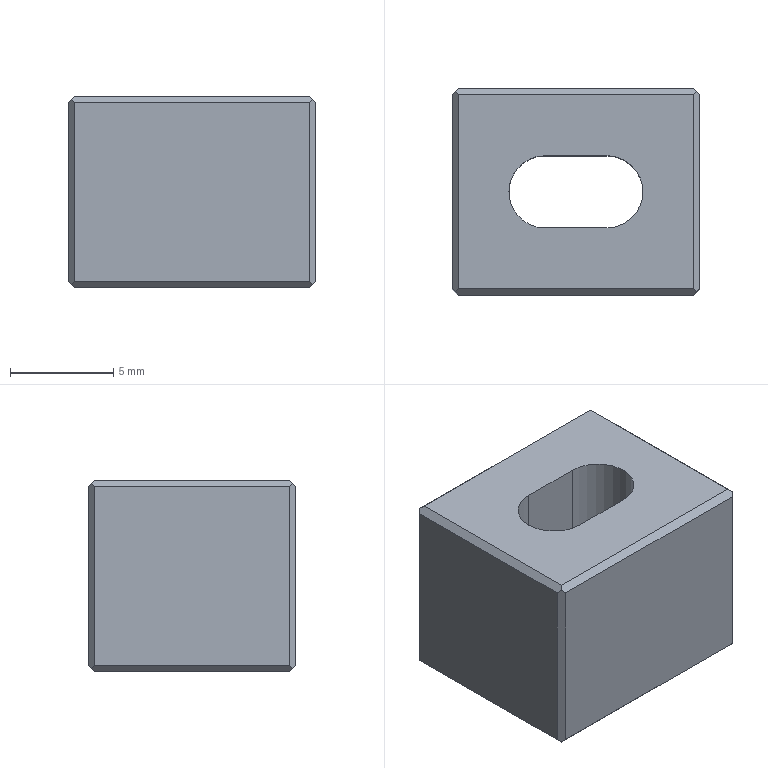Part | NX | 1 solid | 23 faces | box 12 x 10 x 9.3 mm | volume 923.402 mm3 | plane 20 | cylinder 3 | commonest cylinder face diameters 3.5 x3
STEP:
#1=CARTESIAN_POINT('',(-158.2,155.,-51.9));
#2=VERTEX_POINT('',#1);
#3=CARTESIAN_POINT('',(-146.8,155.,-51.9));
#4=VERTEX_POINT('',#3);
#5=CARTESIAN_POINT('',(-152.35,155.,-51.9));
#6=DIRECTION('',(1.,0.,0.));
#7=VECTOR('',#6,1000.);
#8=LINE('',#5,#7);
#9=EDGE_CURVE('',#2,#4,#8,.T.);
#10=ORIENTED_EDGE('',*,*,#9,.T.);
#11=CARTESIAN_POINT('',(-146.8,155.,-43.2));
#12=VERTEX_POINT('',#11);
#13=CARTESIAN_POINT('',(-146.8,155.,-47.55));
#14=DIRECTION('',(0.,0.,1.));
#15=VECTOR('',#14,1000.);
#16=LINE('',#13,#15);
#17=EDGE_CURVE('',#4,#12,#16,.T.);
#18=ORIENTED_EDGE('',*,*,#17,.T.);
#19=CARTESIAN_POINT('',(-158.2,155.,-43.2));
#20=VERTEX_POINT('',#19);
#21=CARTESIAN_POINT('',(-152.5,155.,-43.2));
#22=DIRECTION('',(1.,0.,0.));
#23=VECTOR('',#22,1000.);
#24=LINE('',#21,#23);
#25=EDGE_CURVE('',#20,#12,#24,.T.);
#26=ORIENTED_EDGE('',*,*,#25,.F.);
#27=CARTESIAN_POINT('',(-158.2,155.,-50.566));
#28=DIRECTION('',(0.,0.,1.));
#29=VECTOR('',#28,1000.);
#30=LINE('',#27,#29);
#31=EDGE_CURVE('',#2,#20,#30,.T.);
#32=ORIENTED_EDGE('',*,*,#31,.F.);
#33=EDGE_LOOP('',(#10,#18,#26,#32));
#34=FACE_BOUND('',#33,.T.);
#35=CARTESIAN_POINT('',(-163.5,155.,-58.9));
#36=DIRECTION('',(0.,-1.,0.));
#37=DIRECTION('',(0.,0.,-1.));
#38=AXIS2_PLACEMENT_3D('',#35,#36,#37);
#39=PLANE('',#38);
#40=ADVANCED_FACE('',(#34),#39,.T.);
#41=CARTESIAN_POINT('',(-146.8,164.7,-52.2));
#42=VERTEX_POINT('',#41);
#43=CARTESIAN_POINT('',(-158.2,164.7,-52.2));
#44=VERTEX_POINT('',#43);
#45=CARTESIAN_POINT('',(-152.5,164.7,-52.2));
#46=DIRECTION('',(-1.,0.,0.));
#47=VECTOR('',#46,1000.);
#48=LINE('',#45,#47);
#49=EDGE_CURVE('',#42,#44,#48,.T.);
#50=ORIENTED_EDGE('',*,*,#49,.F.);
#51=CARTESIAN_POINT('',(-146.8,155.3,-52.2));
#52=VERTEX_POINT('',#51);
#53=CARTESIAN_POINT('',(-146.8,159.85,-52.2));
#54=DIRECTION('',(0.,-1.,0.));
#55=VECTOR('',#54,1000.);
#56=LINE('',#53,#55);
#57=EDGE_CURVE('',#42,#52,#56,.T.);
#58=ORIENTED_EDGE('',*,*,#57,.T.);
#59=CARTESIAN_POINT('',(-158.2,155.3,-52.2));
#60=VERTEX_POINT('',#59);
#61=CARTESIAN_POINT('',(-152.35,155.3,-52.2));
#62=DIRECTION('',(1.,0.,0.));
#63=VECTOR('',#62,1000.);
#64=LINE('',#61,#63);
#65=EDGE_CURVE('',#60,#52,#64,.T.);
#66=ORIENTED_EDGE('',*,*,#65,.F.);
#67=CARTESIAN_POINT('',(-158.2,160.,-52.2));
#68=DIRECTION('',(0.,-1.,0.));
#69=VECTOR('',#68,1000.);
#70=LINE('',#67,#69);
#71=EDGE_CURVE('',#44,#60,#70,.T.);
#72=ORIENTED_EDGE('',*,*,#71,.F.);
#73=EDGE_LOOP('',(#50,#58,#66,#72));
#74=FACE_BOUND('',#73,.T.);
#75=CARTESIAN_POINT('',(-154.,158.25,-52.2));
#76=VERTEX_POINT('',#75);
#77=CARTESIAN_POINT('',(-151.,158.25,-52.2));
#78=VERTEX_POINT('',#77);
#79=CARTESIAN_POINT('',(-163.5,158.25,-52.2));
#80=DIRECTION('',(1.,0.,0.));
#81=VECTOR('',#80,1000.);
#82=LINE('',#79,#81);
#83=EDGE_CURVE('',#76,#78,#82,.T.);
#84=ORIENTED_EDGE('',*,*,#83,.T.);
#85=CARTESIAN_POINT('',(-151.,161.75,-52.2));
#86=VERTEX_POINT('',#85);
#87=CARTESIAN_POINT('',(-151.,160.,-52.2));
#88=DIRECTION('',(0.,0.,-1.));
#89=DIRECTION('',(-1.,0.,0.));
#90=AXIS2_PLACEMENT_3D('',#87,#88,#89);
#91=CIRCLE('',#90,1.75);
#92=EDGE_CURVE('',#86,#78,#91,.T.);
#93=ORIENTED_EDGE('',*,*,#92,.F.);
#94=CARTESIAN_POINT('',(-154.,161.75,-52.2));
#95=VERTEX_POINT('',#94);
#96=CARTESIAN_POINT('',(-163.5,161.75,-52.2));
#97=DIRECTION('',(-1.,0.,0.));
#98=VECTOR('',#97,1000.);
#99=LINE('',#96,#98);
#100=EDGE_CURVE('',#86,#95,#99,.T.);
#101=ORIENTED_EDGE('',*,*,#100,.T.);
#102=CARTESIAN_POINT('',(-155.75,160.,-52.2));
#103=VERTEX_POINT('',#102);
#104=CARTESIAN_POINT('',(-154.,160.,-52.2));
#105=DIRECTION('',(0.,0.,-1.));
#106=DIRECTION('',(-1.,0.,0.));
#107=AXIS2_PLACEMENT_3D('',#104,#105,#106);
#108=CIRCLE('',#107,1.75);
#109=EDGE_CURVE('',#103,#95,#108,.T.);
#110=ORIENTED_EDGE('',*,*,#109,.F.);
#111=CARTESIAN_POINT('',(-154.,160.,-52.2));
#112=DIRECTION('',(0.,0.,-1.));
#113=DIRECTION('',(-1.,0.,0.));
#114=AXIS2_PLACEMENT_3D('',#111,#112,#113);
#115=CIRCLE('',#114,1.75);
#116=EDGE_CURVE('',#76,#103,#115,.T.);
#117=ORIENTED_EDGE('',*,*,#116,.F.);
#118=EDGE_LOOP('',(#84,#93,#101,#110,#117));
#119=FACE_BOUND('',#118,.T.);
#120=CARTESIAN_POINT('',(-163.5,162.,-52.2));
#121=DIRECTION('',(0.,0.,-1.));
#122=DIRECTION('',(0.,-1.,0.));
#123=AXIS2_PLACEMENT_3D('',#120,#121,#122);
#124=PLANE('',#123);
#125=ADVANCED_FACE('',(#74,#119),#124,.T.);
#126=CARTESIAN_POINT('',(-146.8,165.,-51.9));
#127=VERTEX_POINT('',#126);
#128=CARTESIAN_POINT('',(-158.2,165.,-51.9));
#129=VERTEX_POINT('',#128);
#130=CARTESIAN_POINT('',(-152.5,165.,-51.9));
#131=DIRECTION('',(-1.,0.,0.));
#132=VECTOR('',#131,1000.);
#133=LINE('',#130,#132);
#134=EDGE_CURVE('',#127,#129,#133,.T.);
#135=ORIENTED_EDGE('',*,*,#134,.T.);
#136=CARTESIAN_POINT('',(-158.2,165.,-43.2));
#137=VERTEX_POINT('',#136);
#138=CARTESIAN_POINT('',(-158.2,165.,-50.566));
#139=DIRECTION('',(0.,0.,-1.));
#140=VECTOR('',#139,1000.);
#141=LINE('',#138,#140);
#142=EDGE_CURVE('',#137,#129,#141,.T.);
#143=ORIENTED_EDGE('',*,*,#142,.F.);
#144=CARTESIAN_POINT('',(-146.8,165.,-43.2));
#145=VERTEX_POINT('',#144);
#146=CARTESIAN_POINT('',(-152.5,165.,-43.2));
#147=DIRECTION('',(-1.,0.,0.));
#148=VECTOR('',#147,1000.);
#149=LINE('',#146,#148);
#150=EDGE_CURVE('',#145,#137,#149,.T.);
#151=ORIENTED_EDGE('',*,*,#150,.F.);
#152=CARTESIAN_POINT('',(-146.8,165.,-50.566));
#153=DIRECTION('',(0.,0.,-1.));
#154=VECTOR('',#153,1000.);
#155=LINE('',#152,#154);
#156=EDGE_CURVE('',#145,#127,#155,.T.);
#157=ORIENTED_EDGE('',*,*,#156,.T.);
#158=EDGE_LOOP('',(#135,#143,#151,#157));
#159=FACE_BOUND('',#158,.T.);
#160=CARTESIAN_POINT('',(-163.5,165.,-42.9));
#161=DIRECTION('',(0.,1.,0.));
#162=DIRECTION('',(1.,0.,0.));
#163=AXIS2_PLACEMENT_3D('',#160,#161,#162);
#164=PLANE('',#163);
#165=ADVANCED_FACE('',(#159),#164,.T.);
#166=CARTESIAN_POINT('',(-158.2,155.3,-42.9));
#167=VERTEX_POINT('',#166);
#168=CARTESIAN_POINT('',(-158.2,164.7,-42.9));
#169=VERTEX_POINT('',#168);
#170=CARTESIAN_POINT('',(-158.2,160.,-42.9));
#171=DIRECTION('',(0.,1.,0.));
#172=VECTOR('',#171,1000.);
#173=LINE('',#170,#172);
#174=EDGE_CURVE('',#167,#169,#173,.T.);
#175=ORIENTED_EDGE('',*,*,#174,.F.);
#176=CARTESIAN_POINT('',(-146.8,155.3,-42.9));
#177=VERTEX_POINT('',#176);
#178=CARTESIAN_POINT('',(-152.5,155.3,-42.9));
#179=DIRECTION('',(1.,0.,0.));
#180=VECTOR('',#179,1000.);
#181=LINE('',#178,#180);
#182=EDGE_CURVE('',#167,#177,#181,.T.);
#183=ORIENTED_EDGE('',*,*,#182,.T.);
#184=CARTESIAN_POINT('',(-146.8,164.7,-42.9));
#185=VERTEX_POINT('',#184);
#186=CARTESIAN_POINT('',(-146.8,160.,-42.9));
#187=DIRECTION('',(0.,1.,0.));
#188=VECTOR('',#187,1000.);
#189=LINE('',#186,#188);
#190=EDGE_CURVE('',#177,#185,#189,.T.);
#191=ORIENTED_EDGE('',*,*,#190,.T.);
#192=CARTESIAN_POINT('',(-152.5,164.7,-42.9));
#193=DIRECTION('',(-1.,0.,0.));
#194=VECTOR('',#193,1000.);
#195=LINE('',#192,#194);
#196=EDGE_CURVE('',#185,#169,#195,.T.);
#197=ORIENTED_EDGE('',*,*,#196,.T.);
#198=EDGE_LOOP('',(#175,#183,#191,#197));
#199=FACE_BOUND('',#198,.T.);
#200=CARTESIAN_POINT('',(-151.,161.75,-42.9));
#201=VERTEX_POINT('',#200);
#202=CARTESIAN_POINT('',(-154.,161.75,-42.9));
#203=VERTEX_POINT('',#202);
#204=CARTESIAN_POINT('',(-163.5,161.75,-42.9));
#205=DIRECTION('',(-1.,0.,0.));
#206=VECTOR('',#205,1000.);
#207=LINE('',#204,#206);
#208=EDGE_CURVE('',#201,#203,#207,.T.);
#209=ORIENTED_EDGE('',*,*,#208,.F.);
#210=CARTESIAN_POINT('',(-151.,158.25,-42.9));
#211=VERTEX_POINT('',#210);
#212=CARTESIAN_POINT('',(-151.,160.,-42.9));
#213=DIRECTION('',(0.,0.,-1.));
#214=DIRECTION('',(-1.,0.,0.));
#215=AXIS2_PLACEMENT_3D('',#212,#213,#214);
#216=CIRCLE('',#215,1.75);
#217=EDGE_CURVE('',#201,#211,#216,.T.);
#218=ORIENTED_EDGE('',*,*,#217,.T.);
#219=CARTESIAN_POINT('',(-154.,158.25,-42.9));
#220=VERTEX_POINT('',#219);
#221=CARTESIAN_POINT('',(-163.5,158.25,-42.9));
#222=DIRECTION('',(1.,0.,0.));
#223=VECTOR('',#222,1000.);
#224=LINE('',#221,#223);
#225=EDGE_CURVE('',#220,#211,#224,.T.);
#226=ORIENTED_EDGE('',*,*,#225,.F.);
#227=CARTESIAN_POINT('',(-155.75,160.,-42.9));
#228=VERTEX_POINT('',#227);
#229=CARTESIAN_POINT('',(-154.,160.,-42.9));
#230=DIRECTION('',(0.,0.,-1.));
#231=DIRECTION('',(-1.,0.,0.));
#232=AXIS2_PLACEMENT_3D('',#229,#230,#231);
#233=CIRCLE('',#232,1.75);
#234=EDGE_CURVE('',#220,#228,#233,.T.);
#235=ORIENTED_EDGE('',*,*,#234,.T.);
#236=CARTESIAN_POINT('',(-154.,160.,-42.9));
#237=DIRECTION('',(0.,0.,-1.));
#238=DIRECTION('',(-1.,0.,0.));
#239=AXIS2_PLACEMENT_3D('',#236,#237,#238);
#240=CIRCLE('',#239,1.75);
#241=EDGE_CURVE('',#228,#203,#240,.T.);
#242=ORIENTED_EDGE('',*,*,#241,.T.);
#243=EDGE_LOOP('',(#209,#218,#226,#235,#242));
#244=FACE_BOUND('',#243,.T.);
#245=CARTESIAN_POINT('',(-163.5,155.8,-42.9));
#246=DIRECTION('',(0.,0.,1.));
#247=DIRECTION('',(1.,0.,0.));
#248=AXIS2_PLACEMENT_3D('',#245,#246,#247);
#249=PLANE('',#248);
#250=ADVANCED_FACE('',(#199,#244),#249,.T.);
#251=CARTESIAN_POINT('',(-155.75,160.,-41.77));
#252=DIRECTION('',(0.,0.,-1.));
#253=VECTOR('',#252,1000.);
#254=LINE('',#251,#253);
#255=EDGE_CURVE('',#228,#103,#254,.T.);
#256=ORIENTED_EDGE('',*,*,#255,.F.);
#257=ORIENTED_EDGE('',*,*,#234,.F.);
#258=CARTESIAN_POINT('',(-154.,158.25,-41.77));
#259=DIRECTION('',(0.,0.,-1.));
#260=VECTOR('',#259,1000.);
#261=LINE('',#258,#260);
#262=EDGE_CURVE('',#220,#76,#261,.T.);
#263=ORIENTED_EDGE('',*,*,#262,.T.);
#264=ORIENTED_EDGE('',*,*,#116,.T.);
#265=EDGE_LOOP('',(#256,#257,#263,#264));
#266=FACE_BOUND('',#265,.T.);
#267=CARTESIAN_POINT('',(-154.,160.,-41.77));
#268=DIRECTION('',(0.,0.,-1.));
#269=DIRECTION('',(-1.,0.,0.));
#270=AXIS2_PLACEMENT_3D('',#267,#268,#269);
#271=CYLINDRICAL_SURFACE('',#270,1.75);
#272=ADVANCED_FACE('',(#266),#271,.F.);
#273=ORIENTED_EDGE('',*,*,#217,.F.);
#274=CARTESIAN_POINT('',(-151.,161.75,-41.77));
#275=DIRECTION('',(0.,0.,-1.));
#276=VECTOR('',#275,1000.);
#277=LINE('',#274,#276);
#278=EDGE_CURVE('',#201,#86,#277,.T.);
#279=ORIENTED_EDGE('',*,*,#278,.T.);
#280=ORIENTED_EDGE('',*,*,#92,.T.);
#281=CARTESIAN_POINT('',(-151.,158.25,-41.77));
#282=DIRECTION('',(0.,0.,-1.));
#283=VECTOR('',#282,1000.);
#284=LINE('',#281,#283);
#285=EDGE_CURVE('',#211,#78,#284,.T.);
#286=ORIENTED_EDGE('',*,*,#285,.F.);
#287=EDGE_LOOP('',(#273,#279,#280,#286));
#288=FACE_BOUND('',#287,.T.);
#289=CARTESIAN_POINT('',(-151.,160.,-41.77));
#290=DIRECTION('',(0.,0.,-1.));
#291=DIRECTION('',(-1.,0.,0.));
#292=AXIS2_PLACEMENT_3D('',#289,#290,#291);
#293=CYLINDRICAL_SURFACE('',#292,1.75);
#294=ADVANCED_FACE('',(#288),#293,.F.);
#295=ORIENTED_EDGE('',*,*,#83,.F.);
#296=ORIENTED_EDGE('',*,*,#262,.F.);
#297=ORIENTED_EDGE('',*,*,#225,.T.);
#298=ORIENTED_EDGE('',*,*,#285,.T.);
#299=EDGE_LOOP('',(#295,#296,#297,#298));
#300=FACE_BOUND('',#299,.T.);
#301=CARTESIAN_POINT('',(-154.,158.25,-41.77));
#302=DIRECTION('',(0.,-1.,0.));
#303=DIRECTION('',(0.,0.,-1.));
#304=AXIS2_PLACEMENT_3D('',#301,#302,#303);
#305=PLANE('',#304);
#306=ADVANCED_FACE('',(#300),#305,.F.);
#307=ORIENTED_EDGE('',*,*,#208,.T.);
#308=CARTESIAN_POINT('',(-154.,161.75,-41.77));
#309=DIRECTION('',(0.,0.,-1.));
#310=VECTOR('',#309,1000.);
#311=LINE('',#308,#310);
#312=EDGE_CURVE('',#203,#95,#311,.T.);
#313=ORIENTED_EDGE('',*,*,#312,.T.);
#314=ORIENTED_EDGE('',*,*,#100,.F.);
#315=ORIENTED_EDGE('',*,*,#278,.F.);
#316=EDGE_LOOP('',(#307,#313,#314,#315));
#317=FACE_BOUND('',#316,.T.);
#318=CARTESIAN_POINT('',(-151.,161.75,-41.77));
#319=DIRECTION('',(0.,1.,0.));
#320=DIRECTION('',(1.,0.,0.));
#321=AXIS2_PLACEMENT_3D('',#318,#319,#320);
#322=PLANE('',#321);
#323=ADVANCED_FACE('',(#317),#322,.F.);
#324=ORIENTED_EDGE('',*,*,#25,.T.);
#325=CARTESIAN_POINT('',(-146.65,155.15,-43.05));
#326=VERTEX_POINT('',#325);
#327=CARTESIAN_POINT('',(-163.5,138.3,-59.9));
#328=DIRECTION('',(-0.5774,-0.5774,-0.5774));
#329=VECTOR('',#328,1000.);
#330=LINE('',#327,#329);
#331=EDGE_CURVE('',#326,#12,#330,.T.);
#332=ORIENTED_EDGE('',*,*,#331,.F.);
#333=CARTESIAN_POINT('',(-163.5,172.,-26.2));
#334=DIRECTION('',(0.5774,-0.5774,-0.5774));
#335=VECTOR('',#334,1000.);
#336=LINE('',#333,#335);
#337=EDGE_CURVE('',#177,#326,#336,.T.);
#338=ORIENTED_EDGE('',*,*,#337,.F.);
#339=ORIENTED_EDGE('',*,*,#182,.F.);
#340=CARTESIAN_POINT('',(-158.35,155.15,-43.05));
#341=VERTEX_POINT('',#340);
#342=CARTESIAN_POINT('',(-165.866,147.634,-50.566));
#343=DIRECTION('',(0.5774,0.5774,0.5774));
#344=VECTOR('',#343,1000.);
#345=LINE('',#342,#344);
#346=EDGE_CURVE('',#341,#167,#345,.T.);
#347=ORIENTED_EDGE('',*,*,#346,.F.);
#348=CARTESIAN_POINT('',(-150.834,147.634,-50.566));
#349=DIRECTION('',(0.5774,-0.5774,-0.5774));
#350=VECTOR('',#349,1000.);
#351=LINE('',#348,#350);
#352=EDGE_CURVE('',#341,#20,#351,.T.);
#353=ORIENTED_EDGE('',*,*,#352,.T.);
#354=EDGE_LOOP('',(#324,#332,#338,#339,#347,#353));
#355=FACE_BOUND('',#354,.T.);
#356=CARTESIAN_POINT('',(-152.5,155.15,-43.05));
#357=DIRECTION('',(0.,0.7071,-0.7071));
#358=DIRECTION('',(-1.,0.,0.));
#359=AXIS2_PLACEMENT_3D('',#356,#357,#358);
#360=PLANE('',#359);
#361=ADVANCED_FACE('',(#355),#360,.F.);
#362=ORIENTED_EDGE('',*,*,#150,.T.);
#363=CARTESIAN_POINT('',(-158.35,164.85,-43.05));
#364=VERTEX_POINT('',#363);
#365=CARTESIAN_POINT('',(-169.713,153.487,-31.687));
#366=DIRECTION('',(0.5774,0.5774,-0.5774));
#367=VECTOR('',#366,1000.);
#368=LINE('',#365,#367);
#369=EDGE_CURVE('',#364,#137,#368,.T.);
#370=ORIENTED_EDGE('',*,*,#369,.F.);
#371=CARTESIAN_POINT('',(-146.987,153.487,-31.687));
#372=DIRECTION('',(-0.5774,0.5774,-0.5774));
#373=VECTOR('',#372,1000.);
#374=LINE('',#371,#373);
#375=EDGE_CURVE('',#169,#364,#374,.T.);
#376=ORIENTED_EDGE('',*,*,#375,.F.);
#377=ORIENTED_EDGE('',*,*,#196,.F.);
#378=CARTESIAN_POINT('',(-146.65,164.85,-43.05));
#379=VERTEX_POINT('',#378);
#380=CARTESIAN_POINT('',(-163.5,148.,-26.2));
#381=DIRECTION('',(-0.5774,-0.5774,0.5774));
#382=VECTOR('',#381,1000.);
#383=LINE('',#380,#382);
#384=EDGE_CURVE('',#379,#185,#383,.T.);
#385=ORIENTED_EDGE('',*,*,#384,.F.);
#386=CARTESIAN_POINT('',(-163.5,181.7,-59.9));
#387=DIRECTION('',(0.5774,-0.5774,0.5774));
#388=VECTOR('',#387,1000.);
#389=LINE('',#386,#388);
#390=EDGE_CURVE('',#145,#379,#389,.T.);
#391=ORIENTED_EDGE('',*,*,#390,.F.);
#392=EDGE_LOOP('',(#362,#370,#376,#377,#385,#391));
#393=FACE_BOUND('',#392,.T.);
#394=CARTESIAN_POINT('',(-152.5,164.85,-43.05));
#395=DIRECTION('',(0.,-0.7071,-0.7071));
#396=DIRECTION('',(0.,-0.7071,0.7071));
#397=AXIS2_PLACEMENT_3D('',#394,#395,#396);
#398=PLANE('',#397);
#399=ADVANCED_FACE('',(#393),#398,.F.);
#400=ORIENTED_EDGE('',*,*,#49,.T.);
#401=CARTESIAN_POINT('',(-158.35,164.85,-52.05));
#402=VERTEX_POINT('',#401);
#403=CARTESIAN_POINT('',(-146.987,153.487,-63.413));
#404=DIRECTION('',(-0.5774,0.5774,0.5774));
#405=VECTOR('',#404,1000.);
#406=LINE('',#403,#405);
#407=EDGE_CURVE('',#44,#402,#406,.T.);
#408=ORIENTED_EDGE('',*,*,#407,.T.);
#409=CARTESIAN_POINT('',(-169.713,153.487,-63.413));
#410=DIRECTION('',(-0.5774,-0.5774,-0.5774));
#411=VECTOR('',#410,1000.);
#412=LINE('',#409,#411);
#413=EDGE_CURVE('',#129,#402,#412,.T.);
#414=ORIENTED_EDGE('',*,*,#413,.F.);
#415=ORIENTED_EDGE('',*,*,#134,.F.);
#416=CARTESIAN_POINT('',(-146.65,164.85,-52.05));
#417=VERTEX_POINT('',#416);
#418=CARTESIAN_POINT('',(-163.5,181.7,-35.2));
#419=DIRECTION('',(0.5774,-0.5774,-0.5774));
#420=VECTOR('',#419,1000.);
#421=LINE('',#418,#420);
#422=EDGE_CURVE('',#127,#417,#421,.T.);
#423=ORIENTED_EDGE('',*,*,#422,.T.);
#424=CARTESIAN_POINT('',(-158.013,153.487,-63.413));
#425=DIRECTION('',(0.5774,0.5774,0.5774));
#426=VECTOR('',#425,1000.);
#427=LINE('',#424,#426);
#428=EDGE_CURVE('',#42,#417,#427,.T.);
#429=ORIENTED_EDGE('',*,*,#428,.F.);
#430=EDGE_LOOP('',(#400,#408,#414,#415,#423,#429));
#431=FACE_BOUND('',#430,.T.);
#432=CARTESIAN_POINT('',(-152.5,164.85,-52.05));
#433=DIRECTION('',(0.,-0.7071,0.7071));
#434=DIRECTION('',(-1.,0.,0.));
#435=AXIS2_PLACEMENT_3D('',#432,#433,#434);
#436=PLANE('',#435);
#437=ADVANCED_FACE('',(#431),#436,.F.);
#438=ORIENTED_EDGE('',*,*,#9,.F.);
#439=CARTESIAN_POINT('',(-158.35,155.15,-52.05));
#440=VERTEX_POINT('',#439);
#441=CARTESIAN_POINT('',(-156.866,153.666,-50.566));
#442=DIRECTION('',(-0.5774,0.5774,-0.5774));
#443=VECTOR('',#442,1000.);
#444=LINE('',#441,#443);
#445=EDGE_CURVE('',#2,#440,#444,.T.);
#446=ORIENTED_EDGE('',*,*,#445,.T.);
#447=CARTESIAN_POINT('',(-159.834,153.666,-50.566));
#448=DIRECTION('',(0.5774,0.5774,-0.5774));
#449=VECTOR('',#448,1000.);
#450=LINE('',#447,#449);
#451=EDGE_CURVE('',#440,#60,#450,.T.);
#452=ORIENTED_EDGE('',*,*,#451,.T.);
#453=ORIENTED_EDGE('',*,*,#65,.T.);
#454=CARTESIAN_POINT('',(-146.65,155.15,-52.05));
#455=VERTEX_POINT('',#454);
#456=CARTESIAN_POINT('',(-163.5,172.,-68.9));
#457=DIRECTION('',(-0.5774,0.5774,-0.5774));
#458=VECTOR('',#457,1000.);
#459=LINE('',#456,#458);
#460=EDGE_CURVE('',#455,#52,#459,.T.);
#461=ORIENTED_EDGE('',*,*,#460,.F.);
#462=CARTESIAN_POINT('',(-163.5,138.3,-35.2));
#463=DIRECTION('',(-0.5774,-0.5774,0.5774));
#464=VECTOR('',#463,1000.);
#465=LINE('',#462,#464);
#466=EDGE_CURVE('',#455,#4,#465,.T.);
#467=ORIENTED_EDGE('',*,*,#466,.T.);
#468=EDGE_LOOP('',(#438,#446,#452,#453,#461,#467));
#469=FACE_BOUND('',#468,.T.);
#470=CARTESIAN_POINT('',(-152.35,155.15,-52.05));
#471=DIRECTION('',(0.,-0.7071,-0.7071));
#472=DIRECTION('',(0.,-0.7071,0.7071));
#473=AXIS2_PLACEMENT_3D('',#470,#471,#472);
#474=PLANE('',#473);
#475=ADVANCED_FACE('',(#469),#474,.T.);
#476=CARTESIAN_POINT('',(-146.5,155.3,-51.9));
#477=VERTEX_POINT('',#476);
#478=CARTESIAN_POINT('',(-146.5,155.3,-43.2));
#479=VERTEX_POINT('',#478);
#480=CARTESIAN_POINT('',(-146.5,155.3,-47.55));
#481=DIRECTION('',(0.,0.,1.));
#482=VECTOR('',#481,1000.);
#483=LINE('',#480,#482);
#484=EDGE_CURVE('',#477,#479,#483,.T.);
#485=ORIENTED_EDGE('',*,*,#484,.F.);
#486=CARTESIAN_POINT('',(-146.5,164.7,-51.9));
#487=VERTEX_POINT('',#486);
#488=CARTESIAN_POINT('',(-146.5,159.85,-51.9));
#489=DIRECTION('',(0.,-1.,0.));
#490=VECTOR('',#489,1000.);
#491=LINE('',#488,#490);
#492=EDGE_CURVE('',#487,#477,#491,.T.);
#493=ORIENTED_EDGE('',*,*,#492,.F.);
#494=CARTESIAN_POINT('',(-146.5,164.7,-43.2));
#495=VERTEX_POINT('',#494);
#496=CARTESIAN_POINT('',(-146.5,164.7,-50.566));
#497=DIRECTION('',(0.,0.,-1.));
#498=VECTOR('',#497,1000.);
#499=LINE('',#496,#498);
#500=EDGE_CURVE('',#495,#487,#499,.T.);
#501=ORIENTED_EDGE('',*,*,#500,.F.);
#502=CARTESIAN_POINT('',(-146.5,160.,-43.2));
#503=DIRECTION('',(0.,1.,0.));
#504=VECTOR('',#503,1000.);
#505=LINE('',#502,#504);
#506=EDGE_CURVE('',#479,#495,#505,.T.);
#507=ORIENTED_EDGE('',*,*,#506,.F.);
#508=EDGE_LOOP('',(#485,#493,#501,#507));
#509=FACE_BOUND('',#508,.T.);
#510=CARTESIAN_POINT('',(-146.5,153.487,-50.566));
#511=DIRECTION('',(-1.,0.,0.));
#512=DIRECTION('',(0.,0.,1.));
#513=AXIS2_PLACEMENT_3D('',#510,#511,#512);
#514=PLANE('',#513);
#515=ADVANCED_FACE('',(#509),#514,.F.);
#516=ORIENTED_EDGE('',*,*,#500,.T.);
#517=CARTESIAN_POINT('',(-163.5,181.7,-68.9));
#518=DIRECTION('',(0.5774,-0.5774,0.5774));
#519=VECTOR('',#518,1000.);
#520=LINE('',#517,#519);
#521=EDGE_CURVE('',#417,#487,#520,.T.);
#522=ORIENTED_EDGE('',*,*,#521,.F.);
#523=ORIENTED_EDGE('',*,*,#422,.F.);
#524=ORIENTED_EDGE('',*,*,#156,.F.);
#525=ORIENTED_EDGE('',*,*,#390,.T.);
#526=CARTESIAN_POINT('',(-163.5,181.7,-26.2));
#527=DIRECTION('',(0.5774,-0.5774,-0.5774));
#528=VECTOR('',#527,1000.);
#529=LINE('',#526,#528);
#530=EDGE_CURVE('',#379,#495,#529,.T.);
#531=ORIENTED_EDGE('',*,*,#530,.T.);
#532=EDGE_LOOP('',(#516,#522,#523,#524,#525,#531));
#533=FACE_BOUND('',#532,.T.);
#534=CARTESIAN_POINT('',(-146.65,164.85,-48.55));
#535=DIRECTION('',(-0.7071,-0.7071,0.));
#536=DIRECTION('',(-0.7071,0.7071,0.));
#537=AXIS2_PLACEMENT_3D('',#534,#535,#536);
#538=PLANE('',#537);
#539=ADVANCED_FACE('',(#533),#538,.F.);
#540=ORIENTED_EDGE('',*,*,#506,.T.);
#541=ORIENTED_EDGE('',*,*,#530,.F.);
#542=ORIENTED_EDGE('',*,*,#384,.T.);
#543=ORIENTED_EDGE('',*,*,#190,.F.);
#544=ORIENTED_EDGE('',*,*,#337,.T.);
#545=CARTESIAN_POINT('',(-163.5,138.3,-26.2));
#546=DIRECTION('',(-0.5774,-0.5774,0.5774));
#547=VECTOR('',#546,1000.);
#548=LINE('',#545,#547);
#549=EDGE_CURVE('',#479,#326,#548,.T.);
#550=ORIENTED_EDGE('',*,*,#549,.F.);
#551=EDGE_LOOP('',(#540,#541,#542,#543,#544,#550));
#552=FACE_BOUND('',#551,.T.);
#553=CARTESIAN_POINT('',(-146.65,160.,-43.05));
#554=DIRECTION('',(-0.7071,0.,-0.7071));
#555=DIRECTION('',(-0.7071,0.,0.7071));
#556=AXIS2_PLACEMENT_3D('',#553,#554,#555);
#557=PLANE('',#556);
#558=ADVANCED_FACE('',(#552),#557,.F.);
#559=ORIENTED_EDGE('',*,*,#492,.T.);
#560=CARTESIAN_POINT('',(-163.5,138.3,-68.9));
#561=DIRECTION('',(0.5774,0.5774,0.5774));
#562=VECTOR('',#561,1000.);
#563=LINE('',#560,#562);
#564=EDGE_CURVE('',#455,#477,#563,.T.);
#565=ORIENTED_EDGE('',*,*,#564,.F.);
#566=ORIENTED_EDGE('',*,*,#460,.T.);
#567=ORIENTED_EDGE('',*,*,#57,.F.);
#568=ORIENTED_EDGE('',*,*,#428,.T.);
#569=ORIENTED_EDGE('',*,*,#521,.T.);
#570=EDGE_LOOP('',(#559,#565,#566,#567,#568,#569));
#571=FACE_BOUND('',#570,.T.);
#572=CARTESIAN_POINT('',(-146.65,159.85,-52.05));
#573=DIRECTION('',(-0.7071,0.,0.7071));
#574=DIRECTION('',(0.,1.,0.));
#575=AXIS2_PLACEMENT_3D('',#572,#573,#574);
#576=PLANE('',#575);
#577=ADVANCED_FACE('',(#571),#576,.F.);
#578=ORIENTED_EDGE('',*,*,#484,.T.);
#579=ORIENTED_EDGE('',*,*,#549,.T.);
#580=ORIENTED_EDGE('',*,*,#331,.T.);
#581=ORIENTED_EDGE('',*,*,#17,.F.);
#582=ORIENTED_EDGE('',*,*,#466,.F.);
#583=ORIENTED_EDGE('',*,*,#564,.T.);
#584=EDGE_LOOP('',(#578,#579,#580,#581,#582,#583));
#585=FACE_BOUND('',#584,.T.);
#586=CARTESIAN_POINT('',(-146.65,155.15,-47.55));
#587=DIRECTION('',(-0.7071,0.7071,0.));
#588=DIRECTION('',(0.,0.,1.));
#589=AXIS2_PLACEMENT_3D('',#586,#587,#588);
#590=PLANE('',#589);
#591=ADVANCED_FACE('',(#585),#590,.F.);
#592=CARTESIAN_POINT('',(-158.5,164.7,-51.9));
#593=VERTEX_POINT('',#592);
#594=CARTESIAN_POINT('',(-158.5,155.3,-51.9));
#595=VERTEX_POINT('',#594);
#596=CARTESIAN_POINT('',(-158.5,160.,-51.9));
#597=DIRECTION('',(0.,-1.,0.));
#598=VECTOR('',#597,1000.);
#599=LINE('',#596,#598);
#600=EDGE_CURVE('',#593,#595,#599,.T.);
#601=ORIENTED_EDGE('',*,*,#600,.T.);
#602=CARTESIAN_POINT('',(-158.5,155.3,-43.2));
#603=VERTEX_POINT('',#602);
#604=CARTESIAN_POINT('',(-158.5,155.3,-50.566));
#605=DIRECTION('',(0.,0.,1.));
#606=VECTOR('',#605,1000.);
#607=LINE('',#604,#606);
#608=EDGE_CURVE('',#595,#603,#607,.T.);
#609=ORIENTED_EDGE('',*,*,#608,.T.);
#610=CARTESIAN_POINT('',(-158.5,164.7,-43.2));
#611=VERTEX_POINT('',#610);
#612=CARTESIAN_POINT('',(-158.5,160.,-43.2));
#613=DIRECTION('',(0.,1.,0.));
#614=VECTOR('',#613,1000.);
#615=LINE('',#612,#614);
#616=EDGE_CURVE('',#603,#611,#615,.T.);
#617=ORIENTED_EDGE('',*,*,#616,.T.);
#618=CARTESIAN_POINT('',(-158.5,164.7,-50.566));
#619=DIRECTION('',(0.,0.,-1.));
#620=VECTOR('',#619,1000.);
#621=LINE('',#618,#620);
#622=EDGE_CURVE('',#611,#593,#621,.T.);
#623=ORIENTED_EDGE('',*,*,#622,.T.);
#624=EDGE_LOOP('',(#601,#609,#617,#623));
#625=FACE_BOUND('',#624,.T.);
#626=CARTESIAN_POINT('',(-158.5,153.487,-50.566));
#627=DIRECTION('',(-1.,0.,0.));
#628=DIRECTION('',(0.,0.,1.));
#629=AXIS2_PLACEMENT_3D('',#626,#627,#628);
#630=PLANE('',#629);
#631=ADVANCED_FACE('',(#625),#630,.T.);
#632=ORIENTED_EDGE('',*,*,#142,.T.);
#633=ORIENTED_EDGE('',*,*,#413,.T.);
#634=CARTESIAN_POINT('',(-169.713,153.487,-40.687));
#635=DIRECTION('',(0.5774,0.5774,-0.5774));
#636=VECTOR('',#635,1000.);
#637=LINE('',#634,#636);
#638=EDGE_CURVE('',#593,#402,#637,.T.);
#639=ORIENTED_EDGE('',*,*,#638,.F.);
#640=ORIENTED_EDGE('',*,*,#622,.F.);
#641=CARTESIAN_POINT('',(-169.713,153.487,-54.413));
#642=DIRECTION('',(0.5774,0.5774,0.5774));
#643=VECTOR('',#642,1000.);
#644=LINE('',#641,#643);
#645=EDGE_CURVE('',#611,#364,#644,.T.);
#646=ORIENTED_EDGE('',*,*,#645,.T.);
#647=ORIENTED_EDGE('',*,*,#369,.T.);
#648=EDGE_LOOP('',(#632,#633,#639,#640,#646,#647));
#649=FACE_BOUND('',#648,.T.);
#650=CARTESIAN_POINT('',(-158.35,164.85,-48.55));
#651=DIRECTION('',(-0.7071,0.7071,0.));
#652=DIRECTION('',(0.,0.,1.));
#653=AXIS2_PLACEMENT_3D('',#650,#651,#652);
#654=PLANE('',#653);
#655=ADVANCED_FACE('',(#649),#654,.T.);
#656=ORIENTED_EDGE('',*,*,#608,.F.);
#657=CARTESIAN_POINT('',(-159.834,156.634,-50.566));
#658=DIRECTION('',(-0.5774,0.5774,0.5774));
#659=VECTOR('',#658,1000.);
#660=LINE('',#657,#659);
#661=EDGE_CURVE('',#440,#595,#660,.T.);
#662=ORIENTED_EDGE('',*,*,#661,.F.);
#663=ORIENTED_EDGE('',*,*,#445,.F.);
#664=ORIENTED_EDGE('',*,*,#31,.T.);
#665=ORIENTED_EDGE('',*,*,#352,.F.);
#666=CARTESIAN_POINT('',(-156.687,153.487,-41.387));
#667=DIRECTION('',(-0.5774,0.5774,-0.5774));
#668=VECTOR('',#667,1000.);
#669=LINE('',#666,#668);
#670=EDGE_CURVE('',#341,#603,#669,.T.);
#671=ORIENTED_EDGE('',*,*,#670,.T.);
#672=EDGE_LOOP('',(#656,#662,#663,#664,#665,#671));
#673=FACE_BOUND('',#672,.T.);
#674=CARTESIAN_POINT('',(-158.35,155.15,-48.55));
#675=DIRECTION('',(-0.7071,-0.7071,0.));
#676=DIRECTION('',(-0.7071,0.7071,0.));
#677=AXIS2_PLACEMENT_3D('',#674,#675,#676);
#678=PLANE('',#677);
#679=ADVANCED_FACE('',(#673),#678,.T.);
#680=ORIENTED_EDGE('',*,*,#616,.F.);
#681=ORIENTED_EDGE('',*,*,#670,.F.);
#682=ORIENTED_EDGE('',*,*,#346,.T.);
#683=ORIENTED_EDGE('',*,*,#174,.T.);
#684=ORIENTED_EDGE('',*,*,#375,.T.);
#685=ORIENTED_EDGE('',*,*,#645,.F.);
#686=EDGE_LOOP('',(#680,#681,#682,#683,#684,#685));
#687=FACE_BOUND('',#686,.T.);
#688=CARTESIAN_POINT('',(-158.35,160.,-43.05));
#689=DIRECTION('',(-0.7071,0.,0.7071));
#690=DIRECTION('',(0.,1.,0.));
#691=AXIS2_PLACEMENT_3D('',#688,#689,#690);
#692=PLANE('',#691);
#693=ADVANCED_FACE('',(#687),#692,.T.);
#694=ORIENTED_EDGE('',*,*,#600,.F.);
#695=ORIENTED_EDGE('',*,*,#638,.T.);
#696=ORIENTED_EDGE('',*,*,#407,.F.);
#697=ORIENTED_EDGE('',*,*,#71,.T.);
#698=ORIENTED_EDGE('',*,*,#451,.F.);
#699=ORIENTED_EDGE('',*,*,#661,.T.);
#700=EDGE_LOOP('',(#694,#695,#696,#697,#698,#699));
#701=FACE_BOUND('',#700,.T.);
#702=CARTESIAN_POINT('',(-158.35,160.,-52.05));
#703=DIRECTION('',(-0.7071,0.,-0.7071));
#704=DIRECTION('',(-0.7071,0.,0.7071));
#705=AXIS2_PLACEMENT_3D('',#702,#703,#704);
#706=PLANE('',#705);
#707=ADVANCED_FACE('',(#701),#706,.T.);
#708=ORIENTED_EDGE('',*,*,#241,.F.);
#709=ORIENTED_EDGE('',*,*,#255,.T.);
#710=ORIENTED_EDGE('',*,*,#109,.T.);
#711=ORIENTED_EDGE('',*,*,#312,.F.);
#712=EDGE_LOOP('',(#708,#709,#710,#711));
#713=FACE_BOUND('',#712,.T.);
#714=CARTESIAN_POINT('',(-154.,160.,-41.77));
#715=DIRECTION('',(0.,0.,-1.));
#716=DIRECTION('',(-1.,0.,0.));
#717=AXIS2_PLACEMENT_3D('',#714,#715,#716);
#718=CYLINDRICAL_SURFACE('',#717,1.75);
#719=ADVANCED_FACE('',(#713),#718,.F.);
#720=CLOSED_SHELL('',(#40,#125,#165,#250,#272,#294,#306,#323,#361,#399,#437,#475,#515,#539,#558,#577,#591,#631,#655,#679,#693,#707,#719));
#721=MANIFOLD_SOLID_BREP('',#720);
#722=(LENGTH_UNIT()NAMED_UNIT(*)SI_UNIT(.MILLI.,.METRE.));
#723=UNCERTAINTY_MEASURE_WITH_UNIT(LENGTH_MEASURE(0.00001),#722,'','');
#724=(NAMED_UNIT(*)PLANE_ANGLE_UNIT()SI_UNIT($,.RADIAN.));
#725=(NAMED_UNIT(*)SI_UNIT($,.STERADIAN.)SOLID_ANGLE_UNIT());
#726=(GEOMETRIC_REPRESENTATION_CONTEXT(3)GLOBAL_UNCERTAINTY_ASSIGNED_CONTEXT((#723))GLOBAL_UNIT_ASSIGNED_CONTEXT((#722,#724,#725))REPRESENTATION_CONTEXT('',''));
#727=ADVANCED_BREP_SHAPE_REPRESENTATION('',(#721),#726);